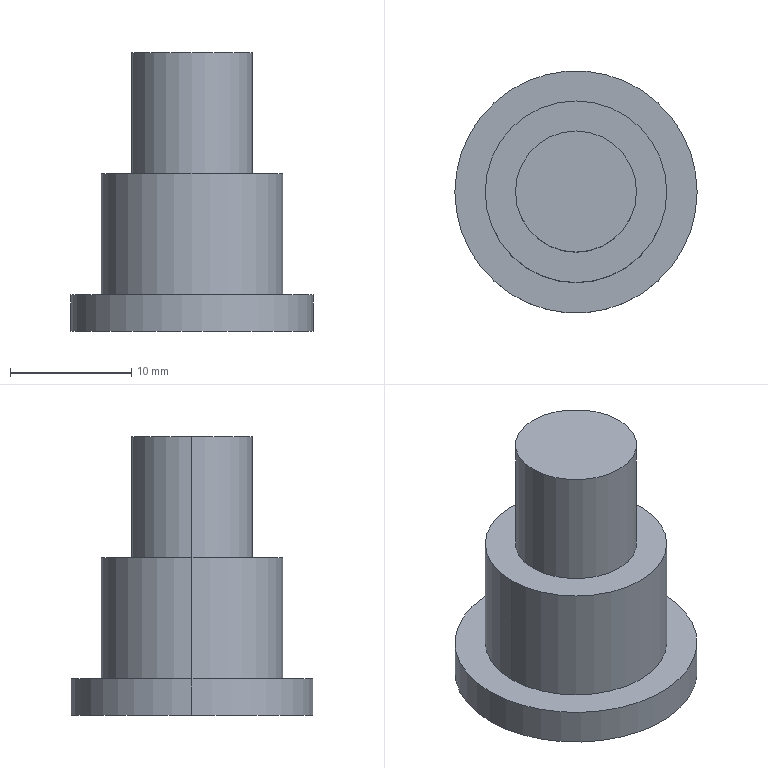Part | SolidWorks | features Revolution 1 | 1 solid | 10 faces | box 20 x 20 x 23 mm | volume 3495 mm3 | cylinder 6 | plane 4 | commonest cylinder face diameters 10 x2 15 x2 20 x2
STEP:
#1=CARTESIAN_POINT('',(5.,0.,-10.));
#2=VERTEX_POINT('',#1);
#3=CARTESIAN_POINT('',(-5.,0.,-10.));
#4=VERTEX_POINT('',#3);
#5=CARTESIAN_POINT('',(0.,0.,-10.));
#6=DIRECTION('',(0.,0.,1.));
#7=DIRECTION('',(1.,0.,0.));
#8=AXIS2_PLACEMENT_3D('',#5,#6,#7);
#9=CIRCLE('',#8,5.);
#10=EDGE_CURVE('',#2,#4,#9,.T.);
#11=ORIENTED_EDGE('',*,*,#10,.T.);
#12=CARTESIAN_POINT('',(-5.,0.,0.));
#13=VERTEX_POINT('',#12);
#14=CARTESIAN_POINT('',(-5.,0.,0.));
#15=DIRECTION('',(0.,0.,1.));
#16=VECTOR('',#15,1000.);
#17=LINE('',#14,#16);
#18=EDGE_CURVE('',#4,#13,#17,.T.);
#19=ORIENTED_EDGE('',*,*,#18,.T.);
#20=CARTESIAN_POINT('',(5.,0.,0.));
#21=VERTEX_POINT('',#20);
#22=CARTESIAN_POINT('',(0.,0.,0.));
#23=DIRECTION('',(0.,0.,1.));
#24=DIRECTION('',(1.,0.,0.));
#25=AXIS2_PLACEMENT_3D('',#22,#23,#24);
#26=CIRCLE('',#25,5.);
#27=EDGE_CURVE('',#21,#13,#26,.T.);
#28=ORIENTED_EDGE('',*,*,#27,.F.);
#29=CARTESIAN_POINT('',(5.,0.,0.));
#30=DIRECTION('',(0.,0.,1.));
#31=VECTOR('',#30,1000.);
#32=LINE('',#29,#31);
#33=EDGE_CURVE('',#2,#21,#32,.T.);
#34=ORIENTED_EDGE('',*,*,#33,.F.);
#35=EDGE_LOOP('',(#11,#19,#28,#34));
#36=FACE_OUTER_BOUND('',#35,.T.);
#37=CARTESIAN_POINT('',(0.,0.,0.));
#38=DIRECTION('',(0.,0.,1.));
#39=DIRECTION('',(1.,0.,0.));
#40=AXIS2_PLACEMENT_3D('',#37,#38,#39);
#41=CYLINDRICAL_SURFACE('',#40,5.);
#42=ADVANCED_FACE('',(#36),#41,.T.);
#43=CARTESIAN_POINT('',(7.5,0.,-20.));
#44=VERTEX_POINT('',#43);
#45=CARTESIAN_POINT('',(-7.5,0.,-20.));
#46=VERTEX_POINT('',#45);
#47=CARTESIAN_POINT('',(0.,0.,-20.));
#48=DIRECTION('',(0.,0.,1.));
#49=DIRECTION('',(1.,0.,0.));
#50=AXIS2_PLACEMENT_3D('',#47,#48,#49);
#51=CIRCLE('',#50,7.5);
#52=EDGE_CURVE('',#44,#46,#51,.T.);
#53=ORIENTED_EDGE('',*,*,#52,.T.);
#54=CARTESIAN_POINT('',(-7.5,0.,-10.));
#55=VERTEX_POINT('',#54);
#56=CARTESIAN_POINT('',(-7.5,0.,0.));
#57=DIRECTION('',(0.,0.,1.));
#58=VECTOR('',#57,1000.);
#59=LINE('',#56,#58);
#60=EDGE_CURVE('',#46,#55,#59,.T.);
#61=ORIENTED_EDGE('',*,*,#60,.T.);
#62=CARTESIAN_POINT('',(7.5,0.,-10.));
#63=VERTEX_POINT('',#62);
#64=CARTESIAN_POINT('',(0.,0.,-10.));
#65=DIRECTION('',(0.,0.,1.));
#66=DIRECTION('',(1.,0.,0.));
#67=AXIS2_PLACEMENT_3D('',#64,#65,#66);
#68=CIRCLE('',#67,7.5);
#69=EDGE_CURVE('',#63,#55,#68,.T.);
#70=ORIENTED_EDGE('',*,*,#69,.F.);
#71=CARTESIAN_POINT('',(7.5,0.,0.));
#72=DIRECTION('',(0.,0.,1.));
#73=VECTOR('',#72,1000.);
#74=LINE('',#71,#73);
#75=EDGE_CURVE('',#44,#63,#74,.T.);
#76=ORIENTED_EDGE('',*,*,#75,.F.);
#77=EDGE_LOOP('',(#53,#61,#70,#76));
#78=FACE_OUTER_BOUND('',#77,.T.);
#79=CARTESIAN_POINT('',(0.,0.,0.));
#80=DIRECTION('',(0.,0.,1.));
#81=DIRECTION('',(1.,0.,0.));
#82=AXIS2_PLACEMENT_3D('',#79,#80,#81);
#83=CYLINDRICAL_SURFACE('',#82,7.5);
#84=ADVANCED_FACE('',(#78),#83,.T.);
#85=CARTESIAN_POINT('',(10.,0.,-23.));
#86=VERTEX_POINT('',#85);
#87=CARTESIAN_POINT('',(-10.,0.,-23.));
#88=VERTEX_POINT('',#87);
#89=CARTESIAN_POINT('',(0.,0.,-23.));
#90=DIRECTION('',(0.,0.,1.));
#91=DIRECTION('',(1.,0.,0.));
#92=AXIS2_PLACEMENT_3D('',#89,#90,#91);
#93=CIRCLE('',#92,10.);
#94=EDGE_CURVE('',#86,#88,#93,.T.);
#95=ORIENTED_EDGE('',*,*,#94,.T.);
#96=CARTESIAN_POINT('',(-10.,0.,-20.));
#97=VERTEX_POINT('',#96);
#98=CARTESIAN_POINT('',(-10.,0.,0.));
#99=DIRECTION('',(0.,0.,1.));
#100=VECTOR('',#99,1000.);
#101=LINE('',#98,#100);
#102=EDGE_CURVE('',#88,#97,#101,.T.);
#103=ORIENTED_EDGE('',*,*,#102,.T.);
#104=CARTESIAN_POINT('',(10.,0.,-20.));
#105=VERTEX_POINT('',#104);
#106=CARTESIAN_POINT('',(0.,0.,-20.));
#107=DIRECTION('',(0.,0.,1.));
#108=DIRECTION('',(1.,0.,0.));
#109=AXIS2_PLACEMENT_3D('',#106,#107,#108);
#110=CIRCLE('',#109,10.);
#111=EDGE_CURVE('',#105,#97,#110,.T.);
#112=ORIENTED_EDGE('',*,*,#111,.F.);
#113=CARTESIAN_POINT('',(10.,0.,0.));
#114=DIRECTION('',(0.,0.,1.));
#115=VECTOR('',#114,1000.);
#116=LINE('',#113,#115);
#117=EDGE_CURVE('',#86,#105,#116,.T.);
#118=ORIENTED_EDGE('',*,*,#117,.F.);
#119=EDGE_LOOP('',(#95,#103,#112,#118));
#120=FACE_OUTER_BOUND('',#119,.T.);
#121=CARTESIAN_POINT('',(0.,0.,0.));
#122=DIRECTION('',(0.,0.,1.));
#123=DIRECTION('',(1.,0.,0.));
#124=AXIS2_PLACEMENT_3D('',#121,#122,#123);
#125=CYLINDRICAL_SURFACE('',#124,10.);
#126=ADVANCED_FACE('',(#120),#125,.T.);
#127=ORIENTED_EDGE('',*,*,#94,.F.);
#128=CARTESIAN_POINT('',(0.,0.,-23.));
#129=DIRECTION('',(0.,0.,1.));
#130=DIRECTION('',(1.,0.,0.));
#131=AXIS2_PLACEMENT_3D('',#128,#129,#130);
#132=CIRCLE('',#131,10.);
#133=EDGE_CURVE('',#88,#86,#132,.T.);
#134=ORIENTED_EDGE('',*,*,#133,.F.);
#135=EDGE_LOOP('',(#127,#134));
#136=FACE_OUTER_BOUND('',#135,.T.);
#137=CARTESIAN_POINT('',(0.,0.,-23.));
#138=DIRECTION('',(0.,0.,1.));
#139=DIRECTION('',(1.,0.,0.));
#140=AXIS2_PLACEMENT_3D('',#137,#138,#139);
#141=PLANE('',#140);
#142=ADVANCED_FACE('',(#136),#141,.F.);
#143=ORIENTED_EDGE('',*,*,#102,.F.);
#144=ORIENTED_EDGE('',*,*,#133,.T.);
#145=ORIENTED_EDGE('',*,*,#117,.T.);
#146=CARTESIAN_POINT('',(0.,0.,-20.));
#147=DIRECTION('',(0.,0.,1.));
#148=DIRECTION('',(1.,0.,0.));
#149=AXIS2_PLACEMENT_3D('',#146,#147,#148);
#150=CIRCLE('',#149,10.);
#151=EDGE_CURVE('',#97,#105,#150,.T.);
#152=ORIENTED_EDGE('',*,*,#151,.F.);
#153=EDGE_LOOP('',(#143,#144,#145,#152));
#154=FACE_OUTER_BOUND('',#153,.T.);
#155=CARTESIAN_POINT('',(0.,0.,0.));
#156=DIRECTION('',(0.,0.,1.));
#157=DIRECTION('',(1.,0.,0.));
#158=AXIS2_PLACEMENT_3D('',#155,#156,#157);
#159=CYLINDRICAL_SURFACE('',#158,10.);
#160=ADVANCED_FACE('',(#154),#159,.T.);
#161=ORIENTED_EDGE('',*,*,#52,.F.);
#162=CARTESIAN_POINT('',(0.,0.,-20.));
#163=DIRECTION('',(0.,0.,1.));
#164=DIRECTION('',(1.,0.,0.));
#165=AXIS2_PLACEMENT_3D('',#162,#163,#164);
#166=CIRCLE('',#165,7.5);
#167=EDGE_CURVE('',#46,#44,#166,.T.);
#168=ORIENTED_EDGE('',*,*,#167,.F.);
#169=EDGE_LOOP('',(#161,#168));
#170=FACE_BOUND('',#169,.T.);
#171=ORIENTED_EDGE('',*,*,#111,.T.);
#172=ORIENTED_EDGE('',*,*,#151,.T.);
#173=EDGE_LOOP('',(#171,#172));
#174=FACE_OUTER_BOUND('',#173,.T.);
#175=CARTESIAN_POINT('',(0.,10.,-20.));
#176=DIRECTION('',(0.,0.,-1.));
#177=DIRECTION('',(-1.,0.,0.));
#178=AXIS2_PLACEMENT_3D('',#175,#176,#177);
#179=PLANE('',#178);
#180=ADVANCED_FACE('',(#170,#174),#179,.F.);
#181=ORIENTED_EDGE('',*,*,#60,.F.);
#182=ORIENTED_EDGE('',*,*,#167,.T.);
#183=ORIENTED_EDGE('',*,*,#75,.T.);
#184=CARTESIAN_POINT('',(0.,0.,-10.));
#185=DIRECTION('',(0.,0.,1.));
#186=DIRECTION('',(1.,0.,0.));
#187=AXIS2_PLACEMENT_3D('',#184,#185,#186);
#188=CIRCLE('',#187,7.5);
#189=EDGE_CURVE('',#55,#63,#188,.T.);
#190=ORIENTED_EDGE('',*,*,#189,.F.);
#191=EDGE_LOOP('',(#181,#182,#183,#190));
#192=FACE_OUTER_BOUND('',#191,.T.);
#193=CARTESIAN_POINT('',(0.,0.,0.));
#194=DIRECTION('',(0.,0.,1.));
#195=DIRECTION('',(1.,0.,0.));
#196=AXIS2_PLACEMENT_3D('',#193,#194,#195);
#197=CYLINDRICAL_SURFACE('',#196,7.5);
#198=ADVANCED_FACE('',(#192),#197,.T.);
#199=ORIENTED_EDGE('',*,*,#10,.F.);
#200=CARTESIAN_POINT('',(0.,0.,-10.));
#201=DIRECTION('',(0.,0.,1.));
#202=DIRECTION('',(1.,0.,0.));
#203=AXIS2_PLACEMENT_3D('',#200,#201,#202);
#204=CIRCLE('',#203,5.);
#205=EDGE_CURVE('',#4,#2,#204,.T.);
#206=ORIENTED_EDGE('',*,*,#205,.F.);
#207=EDGE_LOOP('',(#199,#206));
#208=FACE_BOUND('',#207,.T.);
#209=ORIENTED_EDGE('',*,*,#69,.T.);
#210=ORIENTED_EDGE('',*,*,#189,.T.);
#211=EDGE_LOOP('',(#209,#210));
#212=FACE_OUTER_BOUND('',#211,.T.);
#213=CARTESIAN_POINT('',(0.,5.,-10.));
#214=DIRECTION('',(0.,0.,-1.));
#215=DIRECTION('',(-1.,0.,0.));
#216=AXIS2_PLACEMENT_3D('',#213,#214,#215);
#217=PLANE('',#216);
#218=ADVANCED_FACE('',(#208,#212),#217,.F.);
#219=ORIENTED_EDGE('',*,*,#18,.F.);
#220=ORIENTED_EDGE('',*,*,#205,.T.);
#221=ORIENTED_EDGE('',*,*,#33,.T.);
#222=CARTESIAN_POINT('',(0.,0.,0.));
#223=DIRECTION('',(0.,0.,1.));
#224=DIRECTION('',(1.,0.,0.));
#225=AXIS2_PLACEMENT_3D('',#222,#223,#224);
#226=CIRCLE('',#225,5.);
#227=EDGE_CURVE('',#13,#21,#226,.T.);
#228=ORIENTED_EDGE('',*,*,#227,.F.);
#229=EDGE_LOOP('',(#219,#220,#221,#228));
#230=FACE_OUTER_BOUND('',#229,.T.);
#231=CARTESIAN_POINT('',(0.,0.,0.));
#232=DIRECTION('',(0.,0.,1.));
#233=DIRECTION('',(1.,0.,0.));
#234=AXIS2_PLACEMENT_3D('',#231,#232,#233);
#235=CYLINDRICAL_SURFACE('',#234,5.);
#236=ADVANCED_FACE('',(#230),#235,.T.);
#237=ORIENTED_EDGE('',*,*,#27,.T.);
#238=ORIENTED_EDGE('',*,*,#227,.T.);
#239=EDGE_LOOP('',(#237,#238));
#240=FACE_OUTER_BOUND('',#239,.T.);
#241=CARTESIAN_POINT('',(0.,5.,0.));
#242=DIRECTION('',(0.,0.,-1.));
#243=DIRECTION('',(-1.,0.,0.));
#244=AXIS2_PLACEMENT_3D('',#241,#242,#243);
#245=PLANE('',#244);
#246=ADVANCED_FACE('',(#240),#245,.F.);
#247=CLOSED_SHELL('',(#42,#84,#126,#142,#160,#180,#198,#218,#236,#246));
#248=MANIFOLD_SOLID_BREP('',#247);
#249=CARTESIAN_POINT('',(0.,0.,0.));
#250=DIRECTION('',(0.,0.,1.));
#251=DIRECTION('',(1.,0.,0.));
#252=AXIS2_PLACEMENT_3D('',#249,#250,#251);
#253=(LENGTH_UNIT()NAMED_UNIT(*)SI_UNIT(.MILLI.,.METRE.));
#254=UNCERTAINTY_MEASURE_WITH_UNIT(LENGTH_MEASURE(0.00001),#253,'','');
#255=(NAMED_UNIT(*)PLANE_ANGLE_UNIT()SI_UNIT($,.RADIAN.));
#256=(NAMED_UNIT(*)SI_UNIT($,.STERADIAN.)SOLID_ANGLE_UNIT());
#257=(GEOMETRIC_REPRESENTATION_CONTEXT(3)GLOBAL_UNCERTAINTY_ASSIGNED_CONTEXT((#254))GLOBAL_UNIT_ASSIGNED_CONTEXT((#253,#255,#256))REPRESENTATION_CONTEXT('',''));
#258=ADVANCED_BREP_SHAPE_REPRESENTATION('',(#248,#252),#257);